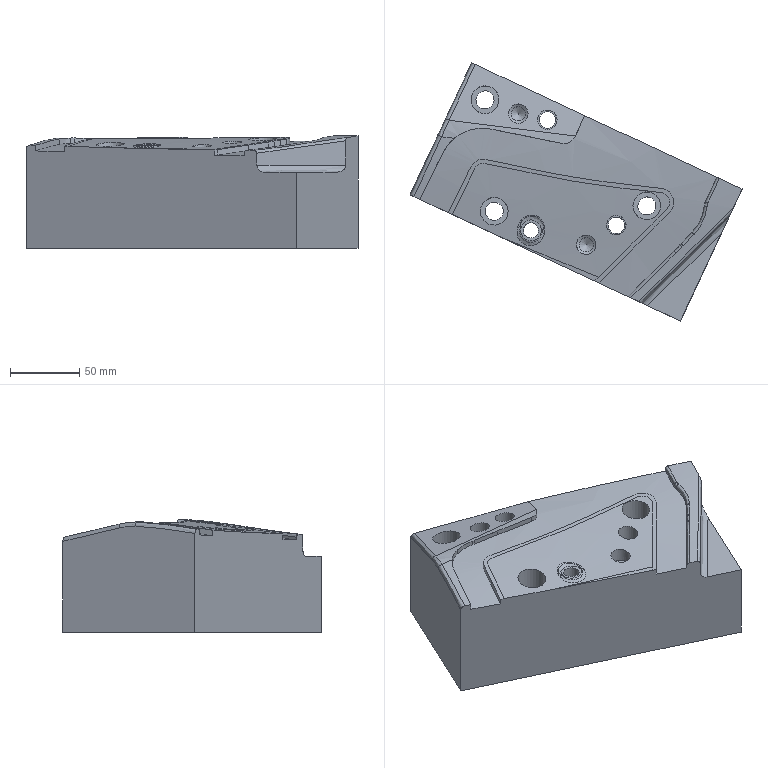Part | STEP file | gslz 2016.10.28-13_id262_x_t | 1 solid | 96 faces | box 239.231 x 186.025 x 81.221 mm | volume 1579297 mm3 | spline 45 | cylinder 17 | other 16 | plane 14 | cone 4 | commonest cylinder face diameters 14 x4 13 x3 20 x3 10.3 x2 12 x2 18 x2